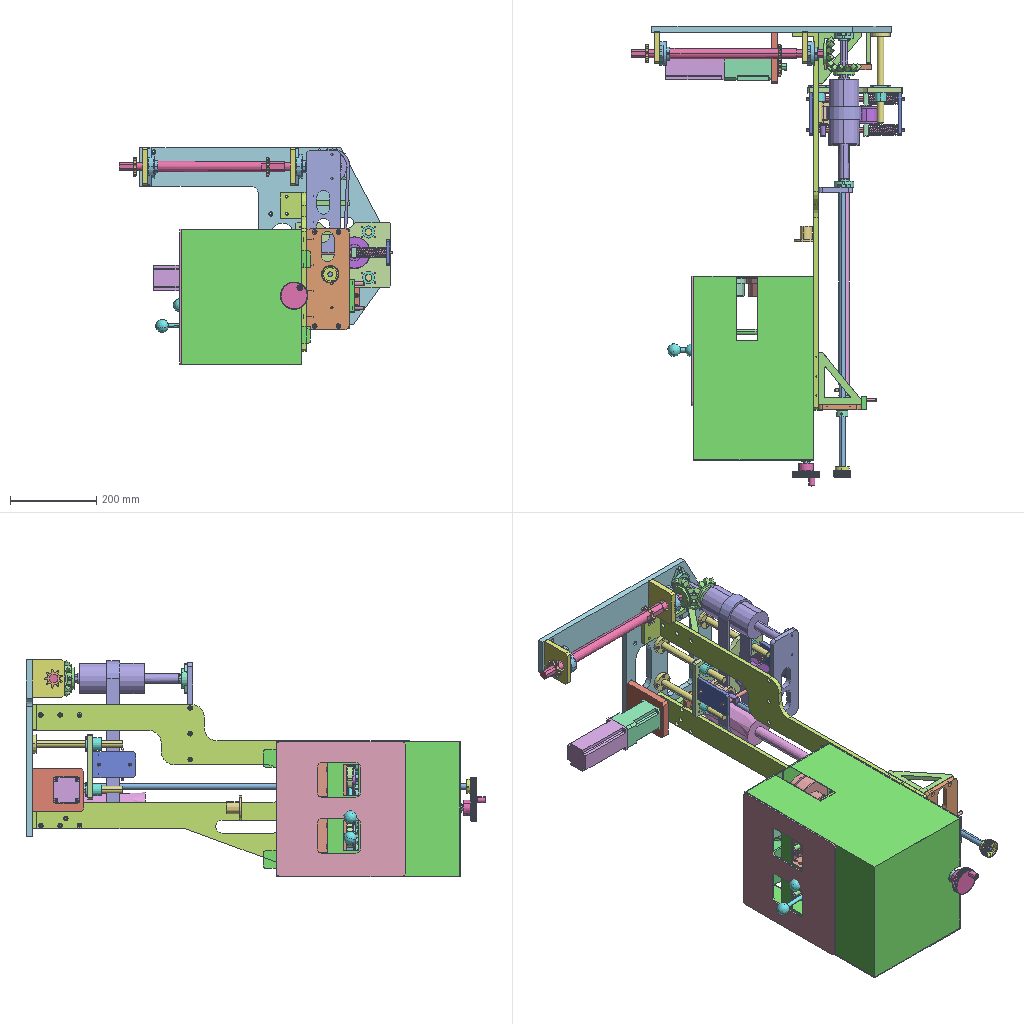Assembly | STEP file | 69 different items | 139 placed | box 635 x 1068 x 505 mm
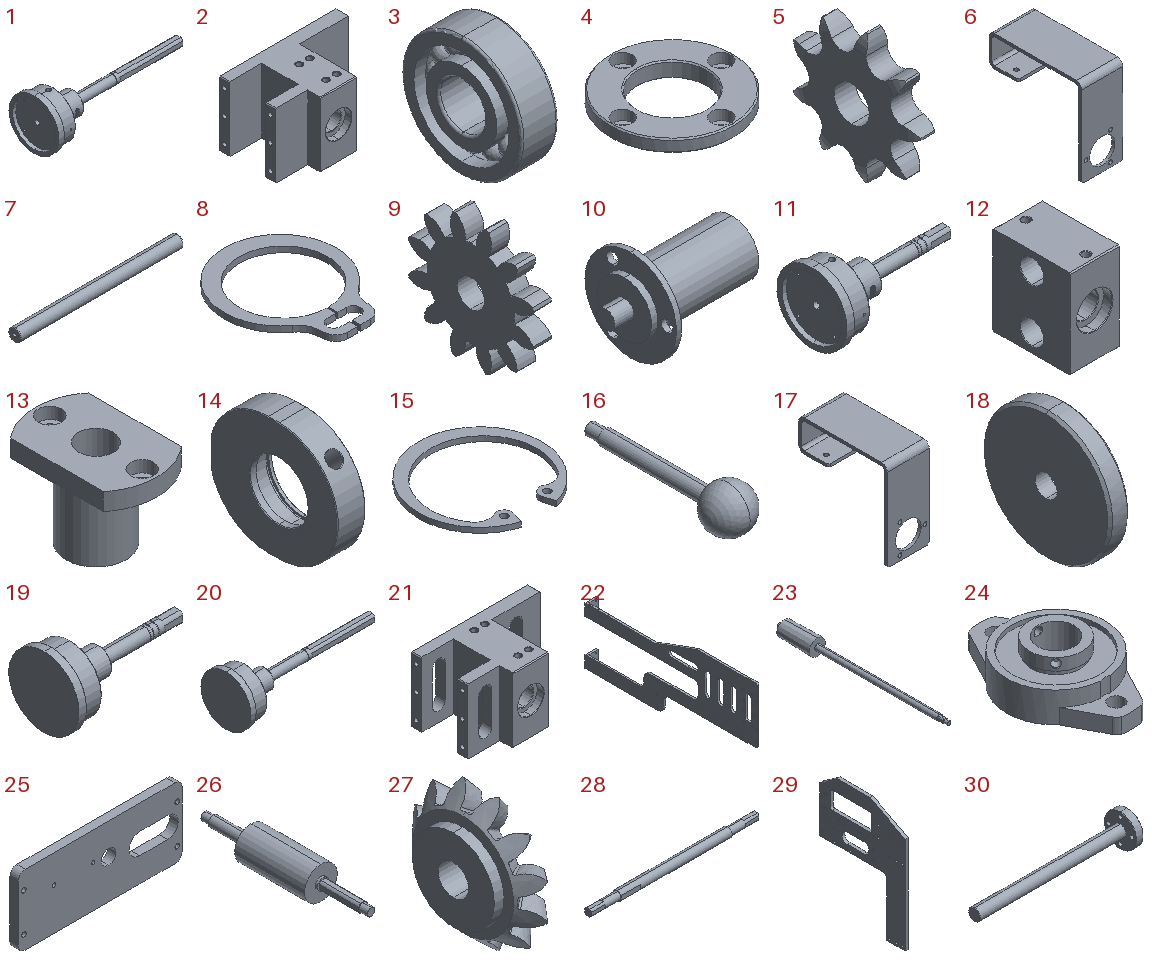Parts list (item | name | quantity | parent item | size | volume):
1 | longitudinal seal wheel 2_SUS304 | x1 | in longitudinal seal fixed shaft assembly | 319 x 110 x 110 mm | 411292 mm3
2 | longitudinal seal bearing seat_SUS304 | x1 | in longitudinal seal fixed shaft assembly | 143.7 x 85 x 80 mm | 392938 mm3
3 | Deep groove ball bearings GB_PreviewCfg | x14 | in longitudinal seal fixed shaft assembly, longitudinal seal movable shaft assembly, opening-closing seat assembly, film pull movable shaft assembly, film pull fixed shaft assembly, adjusting belt tension assembly | 8 x 26 x 26 mm | 2680 mm3
4 | locating sleeve 2 | x2 | in longitudinal seal fixed shaft assembly, film pull fixed shaft assembly | 50 x 50 x 6 mm | 6005 mm3
5 | short pitch roller chain wheel_s_iso_PreviewCfg | x6 | in longitudinal seal fixed shaft assembly, film pull fixed shaft assembly, bevel drive assembly, longitudinal seal film pull assembly 2, servo motor assembly 4 | 7.2 x 43.262 x 43.927 mm | 5700 mm3
6 | rotary joint support_SUS304 | x1 | in longitudinal seal fixed shaft assembly | 44 x 99 x 93 mm | 31796 mm3
7 | 12 small shaft 3_SUS304 | x4 | in longitudinal seal fixed shaft assembly, film pull fixed shaft assembly | 160 x 12 x 12 mm | 17824 mm3
8 | Basic External Retaining Ring_am_PreviewCfg | x12 | in longitudinal seal fixed shaft assembly, longitudinal seal movable shaft assembly, film pull movable shaft assembly, film pull fixed shaft assembly, adjusting belt tension assembly | 4.823 x 5.799 x 0.25 mm | 2.032 mm3
9 | spur gear_iso_PreviewCfg | x4 | in longitudinal seal fixed shaft assembly, longitudinal seal movable shaft assembly, film pull movable shaft assembly, film pull fixed shaft assembly | 12.7 x 86.427 x 86.427 mm | 50526 mm3
10 | SRC025-30 rotary joint_SUS304 | x2 | in longitudinal seal fixed shaft assembly, longitudinal seal movable shaft assembly | 60.7 x 44 x 44 mm | 30292 mm3
11 | longitudinal seal wheel_SUS304 | x1 | in longitudinal seal movable shaft assembly | 209 x 110 x 110 mm | 385908 mm3
12 | longitudinal seal bearing seat 2_SUS304 | x2 | in longitudinal seal movable shaft assembly, film pull movable shaft assembly | 44 x 70 x 80 mm | 178257 mm3
13 | LHFC12_LHFC-12 | x4 | in longitudinal seal movable shaft assembly, film pull movable shaft assembly | 27 x 42 x 30 mm | 10755 mm3
14 | opening-closing seat_SUS304 | x2 | in opening-closing seat assembly | 13 x 59.2 x 55 mm | 24027 mm3
15 | Basic Internal Retaining Ring_am_PreviewCfg | x2 | in opening-closing seat assembly | 26.6 x 26.036 x 1.1 mm | 164.92 mm3
16 | M8 handle_SUS304 | x2 | in opening-closing seat assembly | 30 x 110 x 30 mm | 20164 mm3
17 | rotary joint support 2_SUS304 | x1 | in longitudinal seal movable shaft assembly | 44 x 93 x 93 mm | 30917 mm3
18 | locating ring 6_SUS304 | x4 | in longitudinal seal main assembly, film pull main assembly | 4 x 26 x 26 mm | 1943 mm3
19 | film pull movable wheel_SUS304 | x1 | in film pull movable shaft assembly | 209 x 110 x 110 mm | 448642 mm3
20 | film pull wheel_SUS304 | x1 | in film pull fixed shaft assembly | 319 x 110 x 110 mm | 479492 mm3
21 | longitudinal seal bearing seat 3_SUS304 | x1 | in film pull fixed shaft assembly | 143.7 x 85 x 80 mm | 360424 mm3
22 | longitudinal seal film pull fixing plate_SUS304 | x1 | in longitudinal seal film pull assembly 2 | 60 x 876 x 369 mm | 1562891 mm3
23 | bevel drive wheel_SUS304 | x1 | in bevel drive assembly | 72.6 x 773 x 72.6 mm | 867649 mm3
24 | HBT17_HBT17 | x4 | in bevel drive assembly, bevel drive assembly 3 | 46 x 71 x 19.5 mm | 20624 mm3
25 | support plate 6_SUS304 | x1 | in longitudinal seal film pull assembly 2 | 234 x 12 x 100 mm | 248248 mm3
26 | bevel drive wheel 3_SUS304 | x1 | in bevel drive assembly 3 | 70 x 357 x 70 mm | 643380 mm3
27 | straight miter gear_iso_PreviewCfg | x2 | in miter gear assembly | 25.112 x 82.518 x 82.518 mm | 51040 mm3
28 | shaft 3_SUS304 | x1 | in longitudinal seal film pull assembly 2 | 463.7 x 25 x 25 mm | 196661 mm3
29 | support plate 13_SUS304 | x1 | in longitudinal seal film pull assembly 2 | 14 x 412 x 556 mm | 1475012 mm3
30 | shaft 9_SUS304 | x4 | in longitudinal seal film pull assembly 2 | 210 x 44 x 44 mm | 54427 mm3
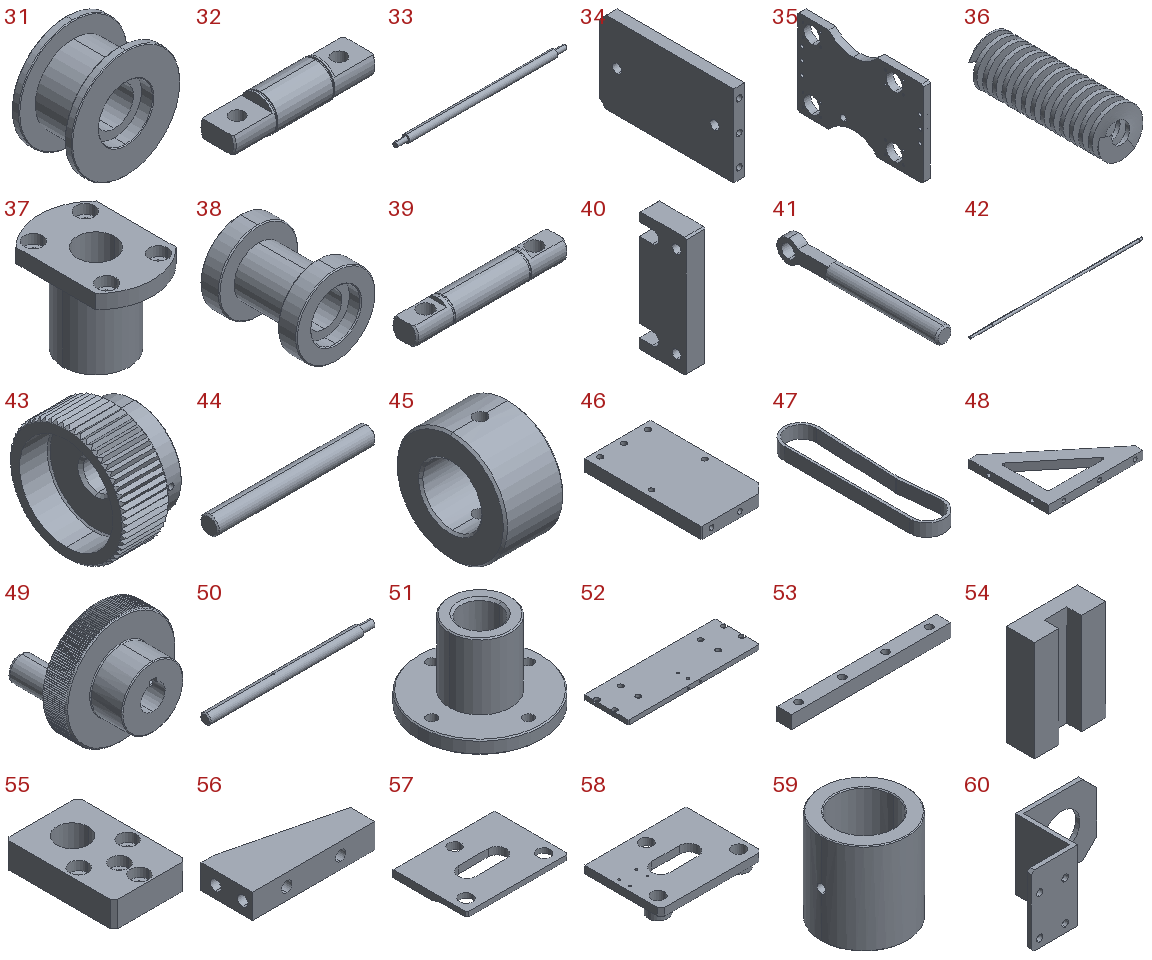31 | adjusting belt tension wheel_SUS304 | x1 | in adjusting belt tension assembly | 74 x 41 x 74 mm | 78222 mm3
32 | tension shaft_SUS304 | x1 | in adjusting belt tension assembly | 100 x 25 x 25 mm | 35682 mm3
33 | sliding shaft_SUS304 | x2 | in adjusting belt tension assembly | 228 x 10 x 10 mm | 16395 mm3
34 | support plate 25_SUS304 | x2 | in adjusting belt tension assembly | 8 x 99 x 60 mm | 46238 mm3
35 | support plate 26_SUS304 | x1 | in adjusting belt tension assembly | 12 x 220 x 150 mm | 331927 mm3
36 | spring 4_SUS304 | x2 | in adjusting belt tension assembly | 24 x 68 x 24 mm | 10180 mm3
37 | LHFC16_LHFC-16 | x4 | in adjusting belt tension assembly | 34 x 48 x 37 mm | 19614 mm3
38 | adjusting belt tension wheel 2_SUS304 | x1 | in adjusting belt tension assembly | 42 x 51 x 42 mm | 27786 mm3
39 | tension shaft 2_SUS304 | x1 | in adjusting belt tension assembly | 100 x 17 x 17 mm | 18904 mm3
40 | support plate 27_SUS304 | x1 | in longitudinal seal film pull assembly 2 | 12 x 30 x 76 mm | 23983 mm3
41 | tension screw_SUS304 | x2 | in longitudinal seal film pull assembly 2 | 8 x 80.6 x 11.2 mm | 3524 mm3
42 | adjusting screw rod 5_SUS304 | x1 | in adjusting screw rod 4 assembly | 950 x 14 x 14 mm | 140280 mm3
43 | KNB12_KNB12 | x1 | in adjusting screw rod 4 assembly | 24 x 40 x 40 mm | 16222 mm3
44 | pin 5_SUS304 | x2 | in adjusting screw rod 4 assembly | 26 x 3 x 3 mm | 183.423 mm3
45 | mounting block_SUS304 | x2 | in adjusting screw rod 4 assembly | 14 x 26 x 26 mm | 5161 mm3
46 | support plate 29 | x1 | in longitudinal seal film pull assembly 2 | 70 x 124 x 12 mm | 100628 mm3
47 | belt 3-4^longitudinal seal film pull assembly 2 | x1 | in longitudinal seal film pull assembly 2 | 82 x 382 x 30 mm | 151088 mm3
48 | reinforcing plate 4 | x4 | in longitudinal seal film pull assembly 2 | 120 x 100 x 10 mm | 45919 mm3
49 | HBK63_HBK63 | x1 | in longitudinal seal height adjusting assembly | 62.998 x 52.8 x 62.995 mm | 59159 mm3
50 | height adjusting screw rod 2A_SUS304 | x1 | in longitudinal seal height adjusting assembly | 326 x 20 x 20 mm | 97813 mm3
51 | adjusting nut 3 | x1 | in longitudinal seal height adjusting assembly | 56 x 56 x 36 mm | 24098 mm3
52 | mounting plate 6 | x1 | in longitudinal seal film pull assembly 2 | 296 x 100 x 10 mm | 288795 mm3
53 | MSA20LE slide rail | x2 | in MSA20LE slide rail assembly | 220 x 20 x 18 mm | 75716 mm3
54 | MSA20LE slide seat | x2 | in MSA20LE slide rail assembly | 63 x 25 x 88.8 mm | 115397 mm3
55 | adjusting nut 4 | x1 | in longitudinal seal film pull assembly 2 | 40 x 60 x 14 mm | 27695 mm3
56 | reinforcing plate 5 | x1 | in longitudinal seal film pull assembly 2 | 50 x 21 x 10 mm | 7392 mm3
57 | support plate 31 | x1 | in longitudinal seal film pull assembly 2 | 170 x 124 x 12 mm | 181853 mm3
58 | support plate 32 | x1 | in longitudinal seal film pull assembly 2 | 164 x 124 x 24 mm | 216301 mm3
59 | locating ring 7 | x1 | in longitudinal seal film pull assembly 2 | 30 x 30 x 32 mm | 11976 mm3
60 | rotary joint support 3.SLDDRW | x1 | in longitudinal seal film pull assembly 2 | 85 x 41.5 x 50 mm | 16429 mm3
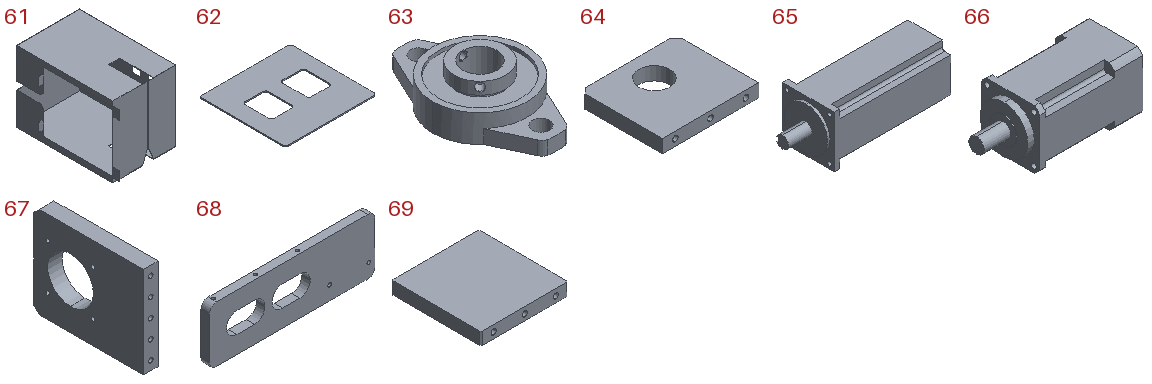61 | cover 10 | x1 | in longitudinal seal film pull assembly 2 | 300 x 458 x 315 mm | 804947 mm3
62 | transparent acrylic | x1 | in longitudinal seal film pull assembly 2 | 315 x 300 x 4 mm | 314343 mm3
63 | HBT20_HBT20 | x2 | in longitudinal seal film pull assembly 2 | 55 x 90 x 23 mm | 35795 mm3
64 | mounting fixed plate | x2 | in longitudinal seal film pull assembly 2 | 88 x 75 x 12 mm | 70480 mm3
65 | MSMD400W-3000 with brake_SUS304 | x1 | in servo motor assembly 4 | 165.5 x 60 x 60 mm | 446542 mm3
66 | AB60-50 (2)_SUS304 | x1 | in servo motor assembly 4 | 145 x 62 x 62 mm | 387545 mm3
67 | servo motor support plate_SUS304 | x1 | in servo motor assembly 4 | 16 x 120 x 100 mm | 157501 mm3
68 | support plate 6A_SUS304 | x1 | in longitudinal seal film pull assembly 2 | 237 x 12 x 80 mm | 190372 mm3
69 | support plate 70 | x1 | in longitudinal seal film pull assembly 2 | 70 x 72 x 10 mm | 49181 mm3
Placements (level | parent | child | x y z in mm | rotation matrix by rows):
1 | longitudinal seal film pull assembly 2 | longitudinal seal main assembly | -657.705 -364.296 -66.725 | -1 0 0 0 -1 0 0 0 1
2 | longitudinal seal main assembly | longitudinal seal fixed shaft assembly | -248.994 -89.603 -0.0 | 1 0 0 0 1 0 0 0 1
3 | longitudinal seal fixed shaft assembly | longitudinal seal wheel 2_SUS304 | -4.608 -14.546 -66.499 | 0 0.8723 0.4889 1 0 0 0 0.4889 -0.8723
3 | longitudinal seal fixed shaft assembly | longitudinal seal bearing seat_SUS304 | -4.608 116.954 -66.499 | 1 0 0 0 1 0 0 0 1
3 | longitudinal seal fixed shaft assembly | Deep groove ball bearings GB_PreviewCfg | -4.608 78.454 -66.499 | 0 -1 0 1 0 0 0 0 1
3 | longitudinal seal fixed shaft assembly | Deep groove ball bearings GB_PreviewCfg | -4.608 155.454 -66.499 | 0 1 0 -1 0 0 0 0 1
3 | longitudinal seal fixed shaft assembly | locating sleeve 2 | -4.608 158.454 -66.499 | 1 0 0 0 0 1 0 -1 -0
3 | longitudinal seal fixed shaft assembly | short pitch roller chain wheel_s_iso_PreviewCfg | -4.608 241.254 -66.499 | 0 -0.3734 0.9277 1 0 0 0 0.9277 0.3734
3 | longitudinal seal fixed shaft assembly | rotary joint support_SUS304 | -4.608 309.954 3.501 | -1 0 0 0 -1 0 0 0 1
3 | longitudinal seal fixed shaft assembly | 12 small shaft 3_SUS304 | -12.608 109.454 -90.499 | 1 0 0 0 1 0 0 0 1
3 | longitudinal seal fixed shaft assembly | 12 small shaft 3_SUS304 | -12.608 109.454 -42.499 | 1 0 0 0 1 0 0 0 1
3 | longitudinal seal fixed shaft assembly | Basic External Retaining Ring_am_PreviewCfg | -4.608 158.454 -66.499 | 1 0 0 0 0 -1 0 1 0
3 | longitudinal seal fixed shaft assembly | spur gear_iso_PreviewCfg | -4.608 178.154 -66.499 | 0 0.3734 0.9277 -1 0 0 0 -0.9277 0.3734
3 | longitudinal seal fixed shaft assembly | SRC025-30 rotary joint_SUS304 | -4.608 295.454 -66.499 | 0 -1 0 1 0 0 0 0 1
2 | longitudinal seal main assembly | longitudinal seal movable shaft assembly | -153.285 -111.536 -143.671 | -1 0 0 0 1 0 0 0 -1
3 | longitudinal seal movable shaft assembly | longitudinal seal wheel_SUS304 | -9.682 7.387 -77.171 | 0 0.8349 -0.5504 1 0 0 0 -0.5504 -0.8349
3 | longitudinal seal movable shaft assembly | longitudinal seal bearing seat 2_SUS304 | -9.682 131.387 -77.171 | 1 0 0 0 1 0 0 0 1
3 | longitudinal seal movable shaft assembly | Deep groove ball bearings GB_PreviewCfg | -9.682 100.387 -77.171 | 0 -1 0 1 0 0 0 0 1
3 | longitudinal seal movable shaft assembly | Deep groove ball bearings GB_PreviewCfg | -9.682 162.387 -77.171 | 0 1 0 -1 0 0 0 0 1
3 | longitudinal seal movable shaft assembly | LHFC12_LHFC-12 | -11.682 131.387 -53.171 | 0 0 1 0 1 0 -1 0 0
3 | longitudinal seal movable shaft assembly | SRC025-30 rotary joint_SUS304 | -9.682 208.387 -77.171 | 0 -1 0 1 0 0 0 0 1
3 | longitudinal seal movable shaft assembly | spur gear_iso_PreviewCfg | -9.682 198.087 -77.171 | 0 0.9594 -0.2822 -1 0 0 0 0.2822 0.9594
3 | longitudinal seal movable shaft assembly | opening-closing seat assembly | -9.065 185.458 -70.895 | 0 -0.09789 -0.9952 1 0 0 0 -0.9952 0.09789
4 | opening-closing seat assembly | opening-closing seat_SUS304 | -18.071 6.307 -0.0 | 1 0 0 0 1 0 0 0 1
4 | opening-closing seat assembly | Deep groove ball bearings GB_PreviewCfg | -11.071 6.307 -0.0 | 1 0 0 0 1 0 0 0 1
4 | opening-closing seat assembly | Basic Internal Retaining Ring_am_PreviewCfg | -6.971 7.113 -0.0 | 0 0 1 0 1 0 -1 0 -0
4 | opening-closing seat assembly | M8 handle_SUS304 | -11.571 -73.243 79.549 | 0.3064 0 -0.9519 0.6731 0.7071 0.2167 0.6731 -0.7071 0.2167
3 | longitudinal seal movable shaft assembly | Basic External Retaining Ring_am_PreviewCfg | -9.682 177.387 -77.171 | 1 0 0 0 0 -1 0 1 -0
3 | longitudinal seal movable shaft assembly | Basic External Retaining Ring_am_PreviewCfg | -9.682 165.387 -77.171 | 1 0 0 0 0 -1 0 1 -0
3 | longitudinal seal movable shaft assembly | Basic External Retaining Ring_am_PreviewCfg | -9.682 169.287 -77.171 | 1 0 0 0 0 -1 0 1 -0
3 | longitudinal seal movable shaft assembly | LHFC12_LHFC-12 | -11.682 131.387 -101.171 | 0 0 1 0 1 0 -1 0 0
3 | longitudinal seal movable shaft assembly | rotary joint support 2_SUS304 | -9.682 222.887 -147.171 | 1 0 0 0 -1 0 0 0 -1
2 | longitudinal seal main assembly | locating ring 6_SUS304 | -98.602 19.85 -42.499 | -1 0 0 0 0.3818 -0.9242 0 -0.9242 -0.3818
2 | longitudinal seal main assembly | locating ring 6_SUS304 | -98.602 19.85 -90.499 | -1 0 0 0 0.3818 -0.9242 0 -0.9242 -0.3818
1 | longitudinal seal film pull assembly 2 | film pull main assembly | -673.894 -339.499 -294.351 | -1 0 0 0 -1 0 0 0 1
2 | film pull main assembly | film pull movable shaft assembly | -143.637 58.452 -24.92 | -1 0 0 0 1 0 0 0 -1
3 | film pull movable shaft assembly | film pull movable wheel_SUS304 | 16.154 -137.805 -56.047 | 0 -0.9376 0.3477 1 0 0 0 0.3477 0.9376
3 | film pull movable shaft assembly | longitudinal seal bearing seat 2_SUS304 | 16.154 -13.805 -56.047 | 1 0 0 0 1 0 0 0 1
3 | film pull movable shaft assembly | Basic External Retaining Ring_am_PreviewCfg | 16.154 32.195 -56.047 | 1 0 0 0 0 -1 0 1 0
3 | film pull movable shaft assembly | Deep groove ball bearings GB_PreviewCfg | 16.154 -44.805 -56.047 | 0 -1 0 1 0 0 0 0 1
3 | film pull movable shaft assembly | Basic External Retaining Ring_am_PreviewCfg | 16.154 24.195 -56.047 | 1 0 0 0 0 -1 0 1 0
3 | film pull movable shaft assembly | Basic External Retaining Ring_am_PreviewCfg | 16.154 21.195 -56.047 | 1 0 0 0 0 -1 0 1 0
3 | film pull movable shaft assembly | Deep groove ball bearings GB_PreviewCfg | 16.154 17.195 -56.047 | 0 1 0 -1 0 0 0 0 1
3 | film pull movable shaft assembly | opening-closing seat assembly | 11.898 39.516 -51.393 | 0 0.6749 -0.7379 1 0 0 0 -0.7379 -0.6749
4 | opening-closing seat assembly | opening-closing seat_SUS304 | -18.071 6.307 -0.0 | 1 0 0 0 1 0 0 0 1
4 | opening-closing seat assembly | Deep groove ball bearings GB_PreviewCfg | -11.071 6.307 -0.0 | 1 0 0 0 1 0 0 0 1
4 | opening-closing seat assembly | Basic Internal Retaining Ring_am_PreviewCfg | -6.971 7.113 -0.0 | 0 0 1 0 1 0 -1 0 -0
4 | opening-closing seat assembly | M8 handle_SUS304 | -11.571 -73.243 79.549 | 0.3064 0 -0.9519 0.6731 0.7071 0.2167 0.6731 -0.7071 0.2167
3 | film pull movable shaft assembly | spur gear_iso_PreviewCfg | 16.154 54.895 -56.047 | 0 0.5473 -0.837 -1 0 0 0 0.837 0.5473
3 | film pull movable shaft assembly | LHFC12_LHFC-12 | 14.154 -13.805 -32.047 | 0 0 1 0 1 0 -1 0 0
3 | film pull movable shaft assembly | LHFC12_LHFC-12 | 14.154 -13.805 -80.047 | 0 0 1 0 1 0 -1 0 0
2 | film pull main assembly | film pull fixed shaft assembly | -245.921 -63.883 92.631 | 1 0 0 0 1 0 0 0 1
3 | film pull fixed shaft assembly | film pull wheel_SUS304 | -23.871 -15.47 -61.504 | 0 0.9498 0.3128 1 0 0 0 0.3128 -0.9498
3 | film pull fixed shaft assembly | longitudinal seal bearing seat 3_SUS304 | -23.871 116.03 -61.504 | 1 0 0 0 1 0 0 0 1
3 | film pull fixed shaft assembly | Deep groove ball bearings GB_PreviewCfg | -23.871 77.53 -61.504 | 0 -1 0 1 0 0 0 0 1
3 | film pull fixed shaft assembly | Deep groove ball bearings GB_PreviewCfg | -23.871 154.53 -61.504 | 0 1 0 -1 0 0 0 0 1
3 | film pull fixed shaft assembly | 12 small shaft 3_SUS304 | -31.871 108.53 -85.504 | 1 0 0 0 1 0 0 0 1
3 | film pull fixed shaft assembly | 12 small shaft 3_SUS304 | -31.871 108.53 -37.504 | 1 0 0 0 1 0 0 0 1
3 | film pull fixed shaft assembly | Basic External Retaining Ring_am_PreviewCfg | -23.871 156.53 -61.504 | 1 0 0 0 0 -1 0 1 0
3 | film pull fixed shaft assembly | spur gear_iso_PreviewCfg | -23.871 177.23 -61.504 | 0 -0.9498 0.3128 -1 0 0 0 -0.3128 -0.9498
3 | film pull fixed shaft assembly | short pitch roller chain wheel_s_iso_PreviewCfg | -23.871 240.33 -61.504 | 0 0.9498 0.3128 1 0 0 0 0.3128 -0.9498
3 | film pull fixed shaft assembly | locating sleeve 2 | -23.871 157.53 -61.504 | 1 0 0 0 0 1 0 -1 -0
2 | film pull main assembly | locating ring 6_SUS304 | -114.791 44.647 55.127 | -1 0 0 0 0.3818 -0.9242 0 -0.9242 -0.3818
2 | film pull main assembly | locating ring 6_SUS304 | -114.791 44.647 7.127 | -1 0 0 0 0.3818 -0.9242 0 -0.9242 -0.3818
1 | longitudinal seal film pull assembly 2 | longitudinal seal film pull fixing plate_SUS304 | -292.103 -316.119 -200.224 | -1 0 0 0 1 0 0 0 -1
1 | longitudinal seal film pull assembly 2 | bevel drive assembly | -232.103 122.104 -130.966 | 0 0 -1 0 1 0 1 0 0
2 | bevel drive assembly | bevel drive wheel_SUS304 | -67.259 -73.37 -0.0 | 1 0 0 0 1 0 0 0 1
2 | bevel drive assembly | short pitch roller chain wheel_s_iso_PreviewCfg | -67.259 -638.051 0.0 | 0 1 0 -1 0 0 0 0 1
2 | bevel drive assembly | HBT17_HBT17 | -67.259 -664.62 -0.0 | 0 1 0 0 0 1 1 0 0
2 | bevel drive assembly | HBT17_HBT17 | -67.259 92.88 0.0 | 0 1 0 0 0 -1 -1 0 -0
1 | longitudinal seal film pull assembly 2 | support plate 6_SUS304 | -292.103 -552.266 -69.224 | 0 0 1 0 -1 0 1 0 -0
1 | longitudinal seal film pull assembly 2 | bevel drive assembly 3 | -268.305 58.135 102.397 | -1 0 0 0 -1 0 0 0 1
2 | bevel drive assembly 3 | bevel drive wheel 3_SUS304 | -36.202 -143.719 -0.6217 | 1 0 0 0 1 0 0 0 1
2 | bevel drive assembly 3 | HBT17_HBT17 | -36.202 -243.969 -0.6217 | 1 0 0 0 0 1 0 -1 -0
2 | bevel drive assembly 3 | HBT17_HBT17 | -36.202 97.531 -0.6217 | -1 0 0 0 0 -1 0 -1 0
2 | bevel drive assembly 3 | miter gear assembly | -20.066 -202.719 -11.393 | -1 0 0 0 0 1 0 1 -0
3 | miter gear assembly | straight miter gear_iso_PreviewCfg | -24.515 10.771 0.0 | 1 0 0 0 1 0 0 0 1
3 | miter gear assembly | straight miter gear_iso_PreviewCfg | 16.136 10.771 40.651 | 0 0 -1 0 -1 0 -1 0 -0
1 | longitudinal seal film pull assembly 2 | shaft 3_SUS304 | -262.191 261.854 101.776 | -1 0 0 0 1 0 0 0 -1
1 | longitudinal seal film pull assembly 2 | short pitch roller chain wheel_s_iso_PreviewCfg | -686.257 261.854 101.776 | -1 0 0 0 -1 0 0 0 1
1 | longitudinal seal film pull assembly 2 | support plate 13_SUS304 | -362.103 325.854 -104.224 | 0 0 1 -1 0 0 0 -1 -0
1 | longitudinal seal film pull assembly 2 | shaft 9_SUS304 | -147.103 101.854 -50.224 | 0 0 -1 1 0 0 0 -1 -0
1 | longitudinal seal film pull assembly 2 | shaft 9_SUS304 | -147.103 101.854 -156.224 | 0 0 -1 1 0 0 0 -1 -0
1 | longitudinal seal film pull assembly 2 | adjusting belt tension assembly | -238.772 145.765 -114.722 | 1 0 0 0 1 0 0 0 1
2 | adjusting belt tension assembly | adjusting belt tension wheel_SUS304 | 58.669 -66.814 16.498 | 1 0 0 0 1 0 0 0 1
2 | adjusting belt tension assembly | Deep groove ball bearings GB_PreviewCfg | 58.669 -9.531 16.498 | 0 -1 0 1 0 0 0 0 1
2 | adjusting belt tension assembly | Deep groove ball bearings GB_PreviewCfg | 58.669 -42.531 16.498 | 0 1 0 -1 0 0 0 0 1
2 | adjusting belt tension assembly | Basic External Retaining Ring_am_PreviewCfg | 58.669 -5.281 16.498 | 1 0 0 0 0 1 0 -1 0
2 | adjusting belt tension assembly | Basic External Retaining Ring_am_PreviewCfg | 58.669 -44.531 16.498 | 1 0 0 0 0 1 0 -1 0
2 | adjusting belt tension assembly | tension shaft_SUS304 | 58.669 -25.031 16.498 | 0 0 -1 1 0 0 0 -1 0
2 | adjusting belt tension assembly | sliding shaft_SUS304 | -65.331 10.969 16.498 | 1 0 0 0 1 0 0 0 1
2 | adjusting belt tension assembly | sliding shaft_SUS304 | -65.331 -61.031 16.498 | 1 0 0 0 1 0 0 0 1
2 | adjusting belt tension assembly | support plate 25_SUS304 | 132.669 -21.031 16.498 | 1 0 0 0 -1 0 0 0 -1
2 | adjusting belt tension assembly | support plate 25_SUS304 | -73.331 -21.031 16.498 | 1 0 0 0 -1 0 0 0 -1
2 | adjusting belt tension assembly | support plate 26_SUS304 | 19.669 24.969 11.498 | 0 -1 0 1 0 0 0 0 1
2 | adjusting belt tension assembly | spring 4_SUS304 | 42.669 10.969 16.498 | 0 1 0 -1 0 0 0 0 1
2 | adjusting belt tension assembly | spring 4_SUS304 | 42.669 -61.031 16.498 | 0 1 0 -1 0 0 0 0 1
2 | adjusting belt tension assembly | LHFC16_LHFC-16 | -52.331 5.969 64.498 | 0 -1 0 0 0 1 -1 0 0
2 | adjusting belt tension assembly | LHFC16_LHFC-16 | 91.669 5.969 64.498 | 0 -1 0 0 0 1 -1 0 0
2 | adjusting belt tension assembly | LHFC16_LHFC-16 | 91.669 5.969 -41.502 | 0 -1 0 0 0 1 -1 0 0
2 | adjusting belt tension assembly | LHFC16_LHFC-16 | -52.331 5.969 -41.502 | 0 -1 0 0 0 1 -1 0 0
2 | adjusting belt tension assembly | adjusting belt tension wheel 2_SUS304 | -41.331 -62.814 16.498 | 1 0 0 0 1 0 0 0 1
2 | adjusting belt tension assembly | Deep groove ball bearings GB_PreviewCfg | -41.331 1.469 16.498 | 0 -1 0 1 0 0 0 0 1
2 | adjusting belt tension assembly | Deep groove ball bearings GB_PreviewCfg | -41.331 -45.531 16.498 | 0 1 0 -1 0 0 0 0 1
2 | adjusting belt tension assembly | Basic External Retaining Ring_am_PreviewCfg | -41.331 -0.2811 16.498 | 1 0 0 0 0 1 0 -1 0
2 | adjusting belt tension assembly | Basic External Retaining Ring_am_PreviewCfg | -41.331 -49.531 16.498 | 1 0 0 0 0 1 0 -1 0
2 | adjusting belt tension assembly | tension shaft 2_SUS304 | -41.331 -25.031 16.498 | 0 0 -1 1 0 0 0 -1 0
1 | longitudinal seal film pull assembly 2 | support plate 27_SUS304 | -192.103 -554.52 -198.224 | 1 0 0 0 1 0 0 0 1
1 | longitudinal seal film pull assembly 2 | tension screw_SUS304 | -232.103 -540.266 -226.224 | 0 -1 0 -1 0 0 0 0 -1
1 | longitudinal seal film pull assembly 2 | tension screw_SUS304 | -232.103 -540.266 -170.224 | 0 -1 0 -1 0 0 0 0 -1
1 | longitudinal seal film pull assembly 2 | shaft 9_SUS304 | -291.103 101.854 -156.224 | 0 0 -1 1 0 0 0 -1 0
1 | longitudinal seal film pull assembly 2 | adjusting screw rod 4 assembly | -144.843 -195.917 -137.085 | 0 -0.992 0.1266 -1 0 0 0 -0.1266 -0.992
2 | adjusting screw rod 4 assembly | adjusting screw rod 5_SUS304 | -428.651 91.936 -0.5 | 1 0 0 0 1 0 0 0 1
2 | adjusting screw rod 4 assembly | KNB12_KNB12 | 525.348 91.936 -0.5 | -1 0 0 0 1 0 0 0 -1
2 | adjusting screw rod 4 assembly | pin 5_SUS304 | 378.349 91.936 -0.5 | 0 0 -1 0 1 0 1 0 -0
2 | adjusting screw rod 4 assembly | mounting block_SUS304 | 352.349 91.936 -0.5 | 1 0 0 0 1 0 0 0 1
2 | adjusting screw rod 4 assembly | mounting block_SUS304 | 378.349 91.936 -0.5 | 1 0 0 0 1 0 0 0 1
2 | adjusting screw rod 4 assembly | pin 5_SUS304 | 352.349 91.936 -0.5 | 0 0 -1 0 1 0 1 0 -0
1 | longitudinal seal film pull assembly 2 | support plate 29 | -230.103 224.734 -198.224 | 0 1 0 0 0 1 1 0 0
1 | longitudinal seal film pull assembly 2 | belt 3-4^longitudinal seal film pull assembly 2 | -232.103 123.734 -198.224 | 1 0 0 0 0 -1 0 1 -0
1 | longitudinal seal film pull assembly 2 | reinforcing plate 4 | -292.103 -552.266 -45.224 | 0 1 0 1 0 0 0 0 -1
1 | longitudinal seal film pull assembly 2 | reinforcing plate 4 | -292.103 311.854 -245.224 | 0 1 0 -1 0 0 0 0 1
1 | longitudinal seal film pull assembly 2 | longitudinal seal height adjusting assembly | -312.146 -695.156 -187.335 | -0.59 0 -0.8074 0 -1 0 -0.8074 0 0.59
2 | longitudinal seal height adjusting assembly | HBK63_HBK63 | 13.487 -6.01 0.0 | 1 0 0 0 1 0 0 0 1
2 | longitudinal seal height adjusting assembly | height adjusting screw rod 2A_SUS304 | 13.487 -309.01 0.0 | 0 0 1 1 0 0 0 1 0
2 | longitudinal seal height adjusting assembly | adjusting nut 3 | 13.487 -520.01 0.0 | 0.4437 0.8962 0 0 0 -1 -0.8962 0.4437 0
1 | longitudinal seal film pull assembly 2 | mounting plate 6 | -332.103 -436.146 -198.224 | 0 0 -1 0 1 0 1 0 0
1 | longitudinal seal film pull assembly 2 | MSA20LE slide rail assembly | -302.103 -363.77 -330.738 | 0 0 -1 -1 0 0 0 1 0
2 | MSA20LE slide rail assembly | MSA20LE slide rail | 16.776 16.014 0.0 | 1 0 0 0 1 0 0 0 1
2 | MSA20LE slide rail assembly | MSA20LE slide seat | 16.776 16.014 7.568 | 0 0 -1 -1 0 0 0 1 0
1 | longitudinal seal film pull assembly 2 | MSA20LE slide rail assembly | -302.103 -363.77 -97.738 | 0 0 -1 -1 0 0 0 1 0
2 | MSA20LE slide rail assembly | MSA20LE slide rail | 16.776 16.014 0.0 | 1 0 0 0 1 0 0 0 1
2 | MSA20LE slide rail assembly | MSA20LE slide seat | 16.776 16.014 7.568 | 0 0 -1 -1 0 0 0 1 0
1 | longitudinal seal film pull assembly 2 | adjusting nut 4 | -333.103 -436.146 -198.224 | 0 1 0 0 0 -1 -1 0 -0
1 | longitudinal seal film pull assembly 2 | reinforcing plate 5 | -342.103 -436.146 -198.224 | 0 -1 0 1 0 0 0 0 1
1 | longitudinal seal film pull assembly 2 | support plate 31 | -364.103 -491.266 -198.224 | 0 1 0 0 0 -1 -1 0 -0
1 | longitudinal seal film pull assembly 2 | support plate 32 | -364.103 -534.147 -198.224 | 0 1 0 0 0 -1 -1 0 -0
1 | longitudinal seal film pull assembly 2 | locating ring 7 | -320.103 -503.266 -198.224 | 1 0 0 0 0 -1 0 1 -0
1 | longitudinal seal film pull assembly 2 | rotary joint support 3.SLDDRW | -344.103 -549.147 -133.224 | -1 0 0 0 -1 0 0 0 1
1 | longitudinal seal film pull assembly 2 | cover 10 | -442.103 -469.146 -358.724 | -1 0 0 0 -1 0 0 0 1
1 | longitudinal seal film pull assembly 2 | transparent acrylic | -582.103 -405.146 -201.224 | 0 0 -1 0 1 0 1 0 -0
1 | longitudinal seal film pull assembly 2 | HBT20_HBT20 | -305.603 261.854 101.776 | 0 0 1 1 0 0 0 1 -0
1 | longitudinal seal film pull assembly 2 | mounting fixed plate | -329.103 275.354 101.776 | 0 0 1 0 -1 0 1 0 -0
1 | longitudinal seal film pull assembly 2 | HBT20_HBT20 | -648.603 261.854 101.776 | 0 0 1 1 0 0 0 1 -0
1 | longitudinal seal film pull assembly 2 | mounting fixed plate | -672.103 275.354 101.776 | 0 0 1 0 -1 0 1 0 -0
1 | longitudinal seal film pull assembly 2 | shaft 9_SUS304 | -291.103 101.854 -50.224 | 0 0 -1 1 0 0 0 -1 -0
1 | longitudinal seal film pull assembly 2 | reinforcing plate 4 | -292.103 311.854 11.776 | 0 1 0 -1 0 0 0 0 1
1 | longitudinal seal film pull assembly 2 | reinforcing plate 4 | -292.103 -552.266 -264.224 | 0 1 0 1 0 0 0 0 -1
1 | longitudinal seal film pull assembly 2 | servo motor assembly 4 | -564.526 230.469 -157.224 | -1 0 0 0 -1 0 0 0 1
2 | servo motor assembly 4 | MSMD400W-3000 with brake_SUS304 | -84.135 -1.385 -0.0 | 1 0 0 0 1 0 0 0 1
2 | servo motor assembly 4 | AB60-50 (2)_SUS304 | -199.135 -1.385 -0.0 | 1 0 0 0 1 0 0 0 1
2 | servo motor assembly 4 | servo motor support plate_SUS304 | -179.135 -21.384 -0.0 | 1 0 0 0 1 0 0 0 1
2 | servo motor assembly 4 | short pitch roller chain wheel_s_iso_PreviewCfg | -179.335 -1.385 0.0 | -1 0 0 0 -0.3818 0.9242 0 0.9242 0.3818
1 | longitudinal seal film pull assembly 2 | short pitch roller chain wheel_s_iso_PreviewCfg | -377.991 261.854 101.776 | -1 0 0 0 1 0 0 0 -1
1 | longitudinal seal film pull assembly 2 | support plate 6A_SUS304 | -212.103 -61.146 -69.224 | 0 0 -1 0 1 0 1 0 0
1 | longitudinal seal film pull assembly 2 | support plate 70 | -170.103 290.35 -198.224 | 0 0 -1 0 1 0 1 0 0